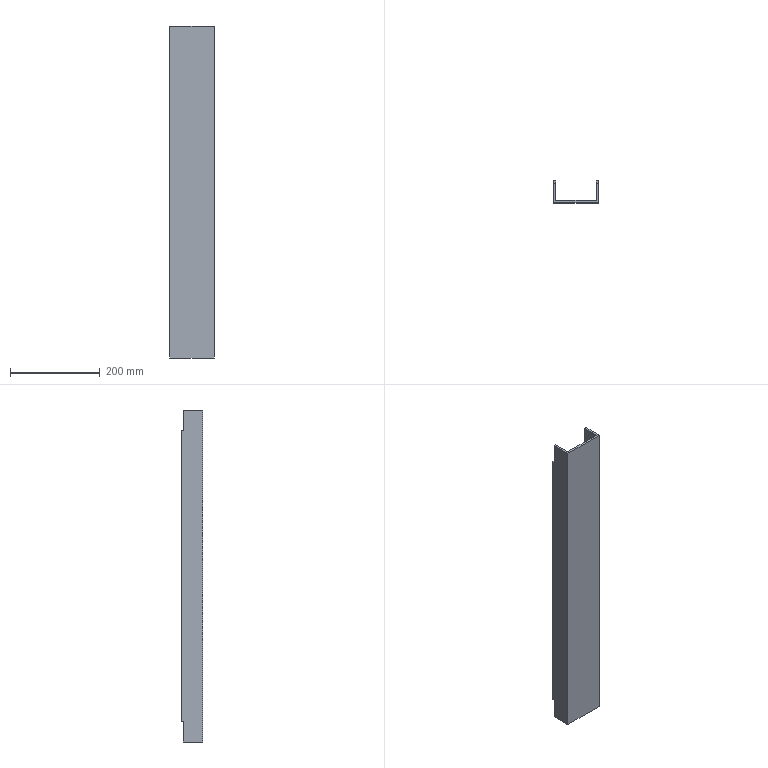Part | SolidWorks | features ICE 6, Cut 4, Extrusion 1 | 1 solid | 18 faces | box 100 x 48 x 740 mm | volume 683700 mm3 | plane 18
STEP:
#1=CARTESIAN_POINT('',(100.,48.,695.));
#2=VERTEX_POINT('',#1);
#3=CARTESIAN_POINT('',(100.,48.,45.));
#4=VERTEX_POINT('',#3);
#5=CARTESIAN_POINT('',(100.,48.,740.));
#6=DIRECTION('',(0.,0.,-1.));
#7=VECTOR('',#6,1000.);
#8=LINE('',#5,#7);
#9=EDGE_CURVE('',#2,#4,#8,.T.);
#10=ORIENTED_EDGE('',*,*,#9,.T.);
#11=CARTESIAN_POINT('',(95.,48.,45.));
#12=VERTEX_POINT('',#11);
#13=CARTESIAN_POINT('',(95.,48.,45.));
#14=DIRECTION('',(1.,0.,0.));
#15=VECTOR('',#14,1000.);
#16=LINE('',#13,#15);
#17=EDGE_CURVE('',#12,#4,#16,.T.);
#18=ORIENTED_EDGE('',*,*,#17,.F.);
#19=CARTESIAN_POINT('',(95.,48.,695.));
#20=VERTEX_POINT('',#19);
#21=CARTESIAN_POINT('',(95.,48.,740.));
#22=DIRECTION('',(0.,0.,-1.));
#23=VECTOR('',#22,1000.);
#24=LINE('',#21,#23);
#25=EDGE_CURVE('',#20,#12,#24,.T.);
#26=ORIENTED_EDGE('',*,*,#25,.F.);
#27=CARTESIAN_POINT('',(100.,48.,695.));
#28=DIRECTION('',(-1.,0.,0.));
#29=VECTOR('',#28,1000.);
#30=LINE('',#27,#29);
#31=EDGE_CURVE('',#2,#20,#30,.T.);
#32=ORIENTED_EDGE('',*,*,#31,.F.);
#33=EDGE_LOOP('',(#10,#18,#26,#32));
#34=FACE_OUTER_BOUND('',#33,.T.);
#35=CARTESIAN_POINT('',(95.,48.,740.));
#36=DIRECTION('',(0.,-1.,0.));
#37=DIRECTION('',(0.,0.,-1.));
#38=AXIS2_PLACEMENT_3D('',#35,#36,#37);
#39=PLANE('',#38);
#40=ADVANCED_FACE('',(#34),#39,.F.);
#41=CARTESIAN_POINT('',(5.,48.,695.));
#42=VERTEX_POINT('',#41);
#43=CARTESIAN_POINT('',(5.,48.,45.));
#44=VERTEX_POINT('',#43);
#45=CARTESIAN_POINT('',(5.,48.,740.));
#46=DIRECTION('',(0.,0.,-1.));
#47=VECTOR('',#46,1000.);
#48=LINE('',#45,#47);
#49=EDGE_CURVE('',#42,#44,#48,.T.);
#50=ORIENTED_EDGE('',*,*,#49,.T.);
#51=CARTESIAN_POINT('',(0.,48.,45.));
#52=VERTEX_POINT('',#51);
#53=CARTESIAN_POINT('',(0.,48.,45.));
#54=DIRECTION('',(1.,0.,0.));
#55=VECTOR('',#54,1000.);
#56=LINE('',#53,#55);
#57=EDGE_CURVE('',#52,#44,#56,.T.);
#58=ORIENTED_EDGE('',*,*,#57,.F.);
#59=CARTESIAN_POINT('',(0.,48.,695.));
#60=VERTEX_POINT('',#59);
#61=CARTESIAN_POINT('',(0.,48.,740.));
#62=DIRECTION('',(0.,0.,-1.));
#63=VECTOR('',#62,1000.);
#64=LINE('',#61,#63);
#65=EDGE_CURVE('',#60,#52,#64,.T.);
#66=ORIENTED_EDGE('',*,*,#65,.F.);
#67=CARTESIAN_POINT('',(5.,48.,695.));
#68=DIRECTION('',(-1.,0.,0.));
#69=VECTOR('',#68,1000.);
#70=LINE('',#67,#69);
#71=EDGE_CURVE('',#42,#60,#70,.T.);
#72=ORIENTED_EDGE('',*,*,#71,.F.);
#73=EDGE_LOOP('',(#50,#58,#66,#72));
#74=FACE_OUTER_BOUND('',#73,.T.);
#75=CARTESIAN_POINT('',(0.,48.,740.));
#76=DIRECTION('',(0.,-1.,0.));
#77=DIRECTION('',(0.,0.,-1.));
#78=AXIS2_PLACEMENT_3D('',#75,#76,#77);
#79=PLANE('',#78);
#80=ADVANCED_FACE('',(#74),#79,.F.);
#81=CARTESIAN_POINT('',(0.,43.,695.));
#82=VERTEX_POINT('',#81);
#83=CARTESIAN_POINT('',(0.,43.,740.));
#84=VERTEX_POINT('',#83);
#85=CARTESIAN_POINT('',(0.,43.,695.));
#86=DIRECTION('',(0.,0.,1.));
#87=VECTOR('',#86,1000.);
#88=LINE('',#85,#87);
#89=EDGE_CURVE('',#82,#84,#88,.T.);
#90=ORIENTED_EDGE('',*,*,#89,.F.);
#91=CARTESIAN_POINT('',(0.,48.,695.));
#92=DIRECTION('',(0.,-1.,0.));
#93=VECTOR('',#92,1000.);
#94=LINE('',#91,#93);
#95=EDGE_CURVE('',#60,#82,#94,.T.);
#96=ORIENTED_EDGE('',*,*,#95,.F.);
#97=ORIENTED_EDGE('',*,*,#65,.T.);
#98=CARTESIAN_POINT('',(0.,43.,45.));
#99=VERTEX_POINT('',#98);
#100=CARTESIAN_POINT('',(0.,43.,45.));
#101=DIRECTION('',(0.,1.,0.));
#102=VECTOR('',#101,1000.);
#103=LINE('',#100,#102);
#104=EDGE_CURVE('',#99,#52,#103,.T.);
#105=ORIENTED_EDGE('',*,*,#104,.F.);
#106=CARTESIAN_POINT('',(0.,43.,0.));
#107=VERTEX_POINT('',#106);
#108=CARTESIAN_POINT('',(0.,43.,45.));
#109=DIRECTION('',(0.,0.,-1.));
#110=VECTOR('',#109,1000.);
#111=LINE('',#108,#110);
#112=EDGE_CURVE('',#99,#107,#111,.T.);
#113=ORIENTED_EDGE('',*,*,#112,.T.);
#114=CARTESIAN_POINT('',(0.,0.,0.));
#115=VERTEX_POINT('',#114);
#116=CARTESIAN_POINT('',(0.,0.,0.));
#117=DIRECTION('',(0.,1.,0.));
#118=VECTOR('',#117,1000.);
#119=LINE('',#116,#118);
#120=EDGE_CURVE('',#115,#107,#119,.T.);
#121=ORIENTED_EDGE('',*,*,#120,.F.);
#122=CARTESIAN_POINT('',(0.,0.,740.));
#123=VERTEX_POINT('',#122);
#124=CARTESIAN_POINT('',(0.,0.,740.));
#125=DIRECTION('',(0.,0.,-1.));
#126=VECTOR('',#125,1000.);
#127=LINE('',#124,#126);
#128=EDGE_CURVE('',#123,#115,#127,.T.);
#129=ORIENTED_EDGE('',*,*,#128,.F.);
#130=CARTESIAN_POINT('',(0.,43.,740.));
#131=DIRECTION('',(0.,-1.,0.));
#132=VECTOR('',#131,1000.);
#133=LINE('',#130,#132);
#134=EDGE_CURVE('',#84,#123,#133,.T.);
#135=ORIENTED_EDGE('',*,*,#134,.F.);
#136=EDGE_LOOP('',(#90,#96,#97,#105,#113,#121,#129,#135));
#137=FACE_OUTER_BOUND('',#136,.T.);
#138=CARTESIAN_POINT('',(0.,0.,740.));
#139=DIRECTION('',(1.,0.,0.));
#140=DIRECTION('',(0.,0.,-1.));
#141=AXIS2_PLACEMENT_3D('',#138,#139,#140);
#142=PLANE('',#141);
#143=ADVANCED_FACE('',(#137),#142,.F.);
#144=CARTESIAN_POINT('',(100.,0.,740.));
#145=VERTEX_POINT('',#144);
#146=CARTESIAN_POINT('',(100.,0.,0.));
#147=VERTEX_POINT('',#146);
#148=CARTESIAN_POINT('',(100.,0.,740.));
#149=DIRECTION('',(0.,0.,-1.));
#150=VECTOR('',#149,1000.);
#151=LINE('',#148,#150);
#152=EDGE_CURVE('',#145,#147,#151,.T.);
#153=ORIENTED_EDGE('',*,*,#152,.F.);
#154=CARTESIAN_POINT('',(0.,0.,740.));
#155=DIRECTION('',(1.,0.,0.));
#156=VECTOR('',#155,1000.);
#157=LINE('',#154,#156);
#158=EDGE_CURVE('',#123,#145,#157,.T.);
#159=ORIENTED_EDGE('',*,*,#158,.F.);
#160=ORIENTED_EDGE('',*,*,#128,.T.);
#161=CARTESIAN_POINT('',(100.,0.,0.));
#162=DIRECTION('',(-1.,0.,0.));
#163=VECTOR('',#162,1000.);
#164=LINE('',#161,#163);
#165=EDGE_CURVE('',#147,#115,#164,.T.);
#166=ORIENTED_EDGE('',*,*,#165,.F.);
#167=EDGE_LOOP('',(#153,#159,#160,#166));
#168=FACE_OUTER_BOUND('',#167,.T.);
#169=CARTESIAN_POINT('',(0.,0.,740.));
#170=DIRECTION('',(0.,1.,0.));
#171=DIRECTION('',(0.,0.,1.));
#172=AXIS2_PLACEMENT_3D('',#169,#170,#171);
#173=PLANE('',#172);
#174=ADVANCED_FACE('',(#168),#173,.F.);
#175=CARTESIAN_POINT('',(100.,43.,695.));
#176=VERTEX_POINT('',#175);
#177=CARTESIAN_POINT('',(100.,43.,695.));
#178=DIRECTION('',(0.,1.,0.));
#179=VECTOR('',#178,1000.);
#180=LINE('',#177,#179);
#181=EDGE_CURVE('',#176,#2,#180,.T.);
#182=ORIENTED_EDGE('',*,*,#181,.F.);
#183=CARTESIAN_POINT('',(100.,43.,740.));
#184=VERTEX_POINT('',#183);
#185=CARTESIAN_POINT('',(100.,43.,695.));
#186=DIRECTION('',(0.,0.,1.));
#187=VECTOR('',#186,1000.);
#188=LINE('',#185,#187);
#189=EDGE_CURVE('',#176,#184,#188,.T.);
#190=ORIENTED_EDGE('',*,*,#189,.T.);
#191=CARTESIAN_POINT('',(100.,0.,740.));
#192=DIRECTION('',(0.,1.,0.));
#193=VECTOR('',#192,1000.);
#194=LINE('',#191,#193);
#195=EDGE_CURVE('',#145,#184,#194,.T.);
#196=ORIENTED_EDGE('',*,*,#195,.F.);
#197=ORIENTED_EDGE('',*,*,#152,.T.);
#198=CARTESIAN_POINT('',(100.,43.,0.));
#199=VERTEX_POINT('',#198);
#200=CARTESIAN_POINT('',(100.,43.,0.));
#201=DIRECTION('',(0.,-1.,0.));
#202=VECTOR('',#201,1000.);
#203=LINE('',#200,#202);
#204=EDGE_CURVE('',#199,#147,#203,.T.);
#205=ORIENTED_EDGE('',*,*,#204,.F.);
#206=CARTESIAN_POINT('',(100.,43.,45.));
#207=VERTEX_POINT('',#206);
#208=CARTESIAN_POINT('',(100.,43.,45.));
#209=DIRECTION('',(0.,0.,-1.));
#210=VECTOR('',#209,1000.);
#211=LINE('',#208,#210);
#212=EDGE_CURVE('',#207,#199,#211,.T.);
#213=ORIENTED_EDGE('',*,*,#212,.F.);
#214=CARTESIAN_POINT('',(100.,48.,45.));
#215=DIRECTION('',(0.,-1.,0.));
#216=VECTOR('',#215,1000.);
#217=LINE('',#214,#216);
#218=EDGE_CURVE('',#4,#207,#217,.T.);
#219=ORIENTED_EDGE('',*,*,#218,.F.);
#220=ORIENTED_EDGE('',*,*,#9,.F.);
#221=EDGE_LOOP('',(#182,#190,#196,#197,#205,#213,#219,#220));
#222=FACE_OUTER_BOUND('',#221,.T.);
#223=CARTESIAN_POINT('',(100.,0.,740.));
#224=DIRECTION('',(-1.,0.,0.));
#225=DIRECTION('',(0.,0.,1.));
#226=AXIS2_PLACEMENT_3D('',#223,#224,#225);
#227=PLANE('',#226);
#228=ADVANCED_FACE('',(#222),#227,.F.);
#229=CARTESIAN_POINT('',(95.,43.,45.));
#230=VERTEX_POINT('',#229);
#231=CARTESIAN_POINT('',(95.,43.,45.));
#232=DIRECTION('',(0.,1.,0.));
#233=VECTOR('',#232,1000.);
#234=LINE('',#231,#233);
#235=EDGE_CURVE('',#230,#12,#234,.T.);
#236=ORIENTED_EDGE('',*,*,#235,.F.);
#237=CARTESIAN_POINT('',(95.,43.,0.));
#238=VERTEX_POINT('',#237);
#239=CARTESIAN_POINT('',(95.,43.,740.));
#240=DIRECTION('',(0.,0.,-1.));
#241=VECTOR('',#240,1000.);
#242=LINE('',#239,#241);
#243=EDGE_CURVE('',#230,#238,#242,.T.);
#244=ORIENTED_EDGE('',*,*,#243,.T.);
#245=CARTESIAN_POINT('',(95.,5.,0.));
#246=VERTEX_POINT('',#245);
#247=CARTESIAN_POINT('',(95.,5.,0.));
#248=DIRECTION('',(0.,1.,0.));
#249=VECTOR('',#248,1000.);
#250=LINE('',#247,#249);
#251=EDGE_CURVE('',#246,#238,#250,.T.);
#252=ORIENTED_EDGE('',*,*,#251,.F.);
#253=CARTESIAN_POINT('',(95.,5.,740.));
#254=VERTEX_POINT('',#253);
#255=CARTESIAN_POINT('',(95.,5.,740.));
#256=DIRECTION('',(0.,0.,-1.));
#257=VECTOR('',#256,1000.);
#258=LINE('',#255,#257);
#259=EDGE_CURVE('',#254,#246,#258,.T.);
#260=ORIENTED_EDGE('',*,*,#259,.F.);
#261=CARTESIAN_POINT('',(95.,43.,740.));
#262=VERTEX_POINT('',#261);
#263=CARTESIAN_POINT('',(95.,43.,740.));
#264=DIRECTION('',(0.,-1.,0.));
#265=VECTOR('',#264,1000.);
#266=LINE('',#263,#265);
#267=EDGE_CURVE('',#262,#254,#266,.T.);
#268=ORIENTED_EDGE('',*,*,#267,.F.);
#269=CARTESIAN_POINT('',(95.,43.,695.));
#270=VERTEX_POINT('',#269);
#271=CARTESIAN_POINT('',(95.,43.,740.));
#272=DIRECTION('',(0.,0.,-1.));
#273=VECTOR('',#272,1000.);
#274=LINE('',#271,#273);
#275=EDGE_CURVE('',#262,#270,#274,.T.);
#276=ORIENTED_EDGE('',*,*,#275,.T.);
#277=CARTESIAN_POINT('',(95.,48.,695.));
#278=DIRECTION('',(0.,-1.,0.));
#279=VECTOR('',#278,1000.);
#280=LINE('',#277,#279);
#281=EDGE_CURVE('',#20,#270,#280,.T.);
#282=ORIENTED_EDGE('',*,*,#281,.F.);
#283=ORIENTED_EDGE('',*,*,#25,.T.);
#284=EDGE_LOOP('',(#236,#244,#252,#260,#268,#276,#282,#283));
#285=FACE_OUTER_BOUND('',#284,.T.);
#286=CARTESIAN_POINT('',(95.,5.,740.));
#287=DIRECTION('',(1.,0.,0.));
#288=DIRECTION('',(0.,0.,-1.));
#289=AXIS2_PLACEMENT_3D('',#286,#287,#288);
#290=PLANE('',#289);
#291=ADVANCED_FACE('',(#285),#290,.F.);
#292=CARTESIAN_POINT('',(5.,5.,740.));
#293=VERTEX_POINT('',#292);
#294=CARTESIAN_POINT('',(5.,5.,0.));
#295=VERTEX_POINT('',#294);
#296=CARTESIAN_POINT('',(5.,5.,740.));
#297=DIRECTION('',(0.,0.,-1.));
#298=VECTOR('',#297,1000.);
#299=LINE('',#296,#298);
#300=EDGE_CURVE('',#293,#295,#299,.T.);
#301=ORIENTED_EDGE('',*,*,#300,.F.);
#302=CARTESIAN_POINT('',(95.,5.,740.));
#303=DIRECTION('',(-1.,0.,0.));
#304=VECTOR('',#303,1000.);
#305=LINE('',#302,#304);
#306=EDGE_CURVE('',#254,#293,#305,.T.);
#307=ORIENTED_EDGE('',*,*,#306,.F.);
#308=ORIENTED_EDGE('',*,*,#259,.T.);
#309=CARTESIAN_POINT('',(5.,5.,0.));
#310=DIRECTION('',(1.,0.,0.));
#311=VECTOR('',#310,1000.);
#312=LINE('',#309,#311);
#313=EDGE_CURVE('',#295,#246,#312,.T.);
#314=ORIENTED_EDGE('',*,*,#313,.F.);
#315=EDGE_LOOP('',(#301,#307,#308,#314));
#316=FACE_OUTER_BOUND('',#315,.T.);
#317=CARTESIAN_POINT('',(5.,5.,740.));
#318=DIRECTION('',(0.,-1.,0.));
#319=DIRECTION('',(0.,0.,-1.));
#320=AXIS2_PLACEMENT_3D('',#317,#318,#319);
#321=PLANE('',#320);
#322=ADVANCED_FACE('',(#316),#321,.F.);
#323=CARTESIAN_POINT('',(5.,43.,695.));
#324=VERTEX_POINT('',#323);
#325=CARTESIAN_POINT('',(5.,43.,695.));
#326=DIRECTION('',(0.,1.,0.));
#327=VECTOR('',#326,1000.);
#328=LINE('',#325,#327);
#329=EDGE_CURVE('',#324,#42,#328,.T.);
#330=ORIENTED_EDGE('',*,*,#329,.F.);
#331=CARTESIAN_POINT('',(5.,43.,740.));
#332=VERTEX_POINT('',#331);
#333=CARTESIAN_POINT('',(5.,43.,740.));
#334=DIRECTION('',(0.,0.,1.));
#335=VECTOR('',#334,1000.);
#336=LINE('',#333,#335);
#337=EDGE_CURVE('',#324,#332,#336,.T.);
#338=ORIENTED_EDGE('',*,*,#337,.T.);
#339=CARTESIAN_POINT('',(5.,5.,740.));
#340=DIRECTION('',(0.,1.,0.));
#341=VECTOR('',#340,1000.);
#342=LINE('',#339,#341);
#343=EDGE_CURVE('',#293,#332,#342,.T.);
#344=ORIENTED_EDGE('',*,*,#343,.F.);
#345=ORIENTED_EDGE('',*,*,#300,.T.);
#346=CARTESIAN_POINT('',(5.,43.,0.));
#347=VERTEX_POINT('',#346);
#348=CARTESIAN_POINT('',(5.,43.,0.));
#349=DIRECTION('',(0.,-1.,0.));
#350=VECTOR('',#349,1000.);
#351=LINE('',#348,#350);
#352=EDGE_CURVE('',#347,#295,#351,.T.);
#353=ORIENTED_EDGE('',*,*,#352,.F.);
#354=CARTESIAN_POINT('',(5.,43.,45.));
#355=VERTEX_POINT('',#354);
#356=CARTESIAN_POINT('',(5.,43.,740.));
#357=DIRECTION('',(0.,0.,1.));
#358=VECTOR('',#357,1000.);
#359=LINE('',#356,#358);
#360=EDGE_CURVE('',#347,#355,#359,.T.);
#361=ORIENTED_EDGE('',*,*,#360,.T.);
#362=CARTESIAN_POINT('',(5.,48.,45.));
#363=DIRECTION('',(0.,-1.,0.));
#364=VECTOR('',#363,1000.);
#365=LINE('',#362,#364);
#366=EDGE_CURVE('',#44,#355,#365,.T.);
#367=ORIENTED_EDGE('',*,*,#366,.F.);
#368=ORIENTED_EDGE('',*,*,#49,.F.);
#369=EDGE_LOOP('',(#330,#338,#344,#345,#353,#361,#367,#368));
#370=FACE_OUTER_BOUND('',#369,.T.);
#371=CARTESIAN_POINT('',(5.,5.,740.));
#372=DIRECTION('',(-1.,0.,0.));
#373=DIRECTION('',(0.,0.,1.));
#374=AXIS2_PLACEMENT_3D('',#371,#372,#373);
#375=PLANE('',#374);
#376=ADVANCED_FACE('',(#370),#375,.F.);
#377=ORIENTED_EDGE('',*,*,#337,.F.);
#378=CARTESIAN_POINT('',(0.,43.,695.));
#379=DIRECTION('',(1.,0.,0.));
#380=VECTOR('',#379,1000.);
#381=LINE('',#378,#380);
#382=EDGE_CURVE('',#82,#324,#381,.T.);
#383=ORIENTED_EDGE('',*,*,#382,.F.);
#384=ORIENTED_EDGE('',*,*,#89,.T.);
#385=CARTESIAN_POINT('',(5.,43.,740.));
#386=DIRECTION('',(-1.,0.,0.));
#387=VECTOR('',#386,1000.);
#388=LINE('',#385,#387);
#389=EDGE_CURVE('',#332,#84,#388,.T.);
#390=ORIENTED_EDGE('',*,*,#389,.F.);
#391=EDGE_LOOP('',(#377,#383,#384,#390));
#392=FACE_OUTER_BOUND('',#391,.T.);
#393=CARTESIAN_POINT('',(0.,43.,695.));
#394=DIRECTION('',(0.,-1.,0.));
#395=DIRECTION('',(0.,0.,-1.));
#396=AXIS2_PLACEMENT_3D('',#393,#394,#395);
#397=PLANE('',#396);
#398=ADVANCED_FACE('',(#392),#397,.F.);
#399=ORIENTED_EDGE('',*,*,#189,.F.);
#400=CARTESIAN_POINT('',(95.,43.,695.));
#401=DIRECTION('',(1.,0.,0.));
#402=VECTOR('',#401,1000.);
#403=LINE('',#400,#402);
#404=EDGE_CURVE('',#270,#176,#403,.T.);
#405=ORIENTED_EDGE('',*,*,#404,.F.);
#406=ORIENTED_EDGE('',*,*,#275,.F.);
#407=CARTESIAN_POINT('',(100.,43.,740.));
#408=DIRECTION('',(-1.,0.,0.));
#409=VECTOR('',#408,1000.);
#410=LINE('',#407,#409);
#411=EDGE_CURVE('',#184,#262,#410,.T.);
#412=ORIENTED_EDGE('',*,*,#411,.F.);
#413=EDGE_LOOP('',(#399,#405,#406,#412));
#414=FACE_OUTER_BOUND('',#413,.T.);
#415=CARTESIAN_POINT('',(0.,43.,695.));
#416=DIRECTION('',(0.,-1.,0.));
#417=DIRECTION('',(0.,0.,-1.));
#418=AXIS2_PLACEMENT_3D('',#415,#416,#417);
#419=PLANE('',#418);
#420=ADVANCED_FACE('',(#414),#419,.F.);
#421=ORIENTED_EDGE('',*,*,#112,.F.);
#422=CARTESIAN_POINT('',(5.,43.,45.));
#423=DIRECTION('',(-1.,0.,0.));
#424=VECTOR('',#423,1000.);
#425=LINE('',#422,#424);
#426=EDGE_CURVE('',#355,#99,#425,.T.);
#427=ORIENTED_EDGE('',*,*,#426,.F.);
#428=ORIENTED_EDGE('',*,*,#360,.F.);
#429=CARTESIAN_POINT('',(0.,43.,0.));
#430=DIRECTION('',(1.,0.,0.));
#431=VECTOR('',#430,1000.);
#432=LINE('',#429,#431);
#433=EDGE_CURVE('',#107,#347,#432,.T.);
#434=ORIENTED_EDGE('',*,*,#433,.F.);
#435=EDGE_LOOP('',(#421,#427,#428,#434));
#436=FACE_OUTER_BOUND('',#435,.T.);
#437=CARTESIAN_POINT('',(100.,43.,45.));
#438=DIRECTION('',(0.,-1.,0.));
#439=DIRECTION('',(0.,0.,-1.));
#440=AXIS2_PLACEMENT_3D('',#437,#438,#439);
#441=PLANE('',#440);
#442=ADVANCED_FACE('',(#436),#441,.F.);
#443=ORIENTED_EDGE('',*,*,#243,.F.);
#444=CARTESIAN_POINT('',(100.,43.,45.));
#445=DIRECTION('',(-1.,0.,0.));
#446=VECTOR('',#445,1000.);
#447=LINE('',#444,#446);
#448=EDGE_CURVE('',#207,#230,#447,.T.);
#449=ORIENTED_EDGE('',*,*,#448,.F.);
#450=ORIENTED_EDGE('',*,*,#212,.T.);
#451=CARTESIAN_POINT('',(95.,43.,0.));
#452=DIRECTION('',(1.,0.,0.));
#453=VECTOR('',#452,1000.);
#454=LINE('',#451,#453);
#455=EDGE_CURVE('',#238,#199,#454,.T.);
#456=ORIENTED_EDGE('',*,*,#455,.F.);
#457=EDGE_LOOP('',(#443,#449,#450,#456));
#458=FACE_OUTER_BOUND('',#457,.T.);
#459=CARTESIAN_POINT('',(100.,43.,45.));
#460=DIRECTION('',(0.,-1.,0.));
#461=DIRECTION('',(0.,0.,-1.));
#462=AXIS2_PLACEMENT_3D('',#459,#460,#461);
#463=PLANE('',#462);
#464=ADVANCED_FACE('',(#458),#463,.F.);
#465=ORIENTED_EDGE('',*,*,#313,.T.);
#466=ORIENTED_EDGE('',*,*,#251,.T.);
#467=ORIENTED_EDGE('',*,*,#455,.T.);
#468=ORIENTED_EDGE('',*,*,#204,.T.);
#469=ORIENTED_EDGE('',*,*,#165,.T.);
#470=ORIENTED_EDGE('',*,*,#120,.T.);
#471=ORIENTED_EDGE('',*,*,#433,.T.);
#472=ORIENTED_EDGE('',*,*,#352,.T.);
#473=EDGE_LOOP('',(#465,#466,#467,#468,#469,#470,#471,#472));
#474=FACE_OUTER_BOUND('',#473,.T.);
#475=CARTESIAN_POINT('',(0.,0.,0.));
#476=DIRECTION('',(0.,0.,1.));
#477=DIRECTION('',(1.,0.,0.));
#478=AXIS2_PLACEMENT_3D('',#475,#476,#477);
#479=PLANE('',#478);
#480=ADVANCED_FACE('',(#474),#479,.F.);
#481=ORIENTED_EDGE('',*,*,#104,.T.);
#482=ORIENTED_EDGE('',*,*,#57,.T.);
#483=ORIENTED_EDGE('',*,*,#366,.T.);
#484=ORIENTED_EDGE('',*,*,#426,.T.);
#485=EDGE_LOOP('',(#481,#482,#483,#484));
#486=FACE_OUTER_BOUND('',#485,.T.);
#487=CARTESIAN_POINT('',(0.,0.,45.));
#488=DIRECTION('',(0.,0.,-1.));
#489=DIRECTION('',(-1.,0.,0.));
#490=AXIS2_PLACEMENT_3D('',#487,#488,#489);
#491=PLANE('',#490);
#492=ADVANCED_FACE('',(#486),#491,.T.);
#493=ORIENTED_EDGE('',*,*,#218,.T.);
#494=ORIENTED_EDGE('',*,*,#448,.T.);
#495=ORIENTED_EDGE('',*,*,#235,.T.);
#496=ORIENTED_EDGE('',*,*,#17,.T.);
#497=EDGE_LOOP('',(#493,#494,#495,#496));
#498=FACE_OUTER_BOUND('',#497,.T.);
#499=CARTESIAN_POINT('',(0.,0.,45.));
#500=DIRECTION('',(0.,0.,-1.));
#501=DIRECTION('',(-1.,0.,0.));
#502=AXIS2_PLACEMENT_3D('',#499,#500,#501);
#503=PLANE('',#502);
#504=ADVANCED_FACE('',(#498),#503,.T.);
#505=ORIENTED_EDGE('',*,*,#134,.T.);
#506=ORIENTED_EDGE('',*,*,#158,.T.);
#507=ORIENTED_EDGE('',*,*,#195,.T.);
#508=ORIENTED_EDGE('',*,*,#411,.T.);
#509=ORIENTED_EDGE('',*,*,#267,.T.);
#510=ORIENTED_EDGE('',*,*,#306,.T.);
#511=ORIENTED_EDGE('',*,*,#343,.T.);
#512=ORIENTED_EDGE('',*,*,#389,.T.);
#513=EDGE_LOOP('',(#505,#506,#507,#508,#509,#510,#511,#512));
#514=FACE_OUTER_BOUND('',#513,.T.);
#515=CARTESIAN_POINT('',(0.,0.,740.));
#516=DIRECTION('',(0.,0.,1.));
#517=DIRECTION('',(1.,0.,0.));
#518=AXIS2_PLACEMENT_3D('',#515,#516,#517);
#519=PLANE('',#518);
#520=ADVANCED_FACE('',(#514),#519,.T.);
#521=ORIENTED_EDGE('',*,*,#95,.T.);
#522=ORIENTED_EDGE('',*,*,#382,.T.);
#523=ORIENTED_EDGE('',*,*,#329,.T.);
#524=ORIENTED_EDGE('',*,*,#71,.T.);
#525=EDGE_LOOP('',(#521,#522,#523,#524));
#526=FACE_OUTER_BOUND('',#525,.T.);
#527=CARTESIAN_POINT('',(0.,0.,695.));
#528=DIRECTION('',(0.,0.,1.));
#529=DIRECTION('',(1.,0.,0.));
#530=AXIS2_PLACEMENT_3D('',#527,#528,#529);
#531=PLANE('',#530);
#532=ADVANCED_FACE('',(#526),#531,.T.);
#533=ORIENTED_EDGE('',*,*,#181,.T.);
#534=ORIENTED_EDGE('',*,*,#31,.T.);
#535=ORIENTED_EDGE('',*,*,#281,.T.);
#536=ORIENTED_EDGE('',*,*,#404,.T.);
#537=EDGE_LOOP('',(#533,#534,#535,#536));
#538=FACE_OUTER_BOUND('',#537,.T.);
#539=CARTESIAN_POINT('',(0.,0.,695.));
#540=DIRECTION('',(0.,0.,1.));
#541=DIRECTION('',(1.,0.,0.));
#542=AXIS2_PLACEMENT_3D('',#539,#540,#541);
#543=PLANE('',#542);
#544=ADVANCED_FACE('',(#538),#543,.T.);
#545=CLOSED_SHELL('',(#40,#80,#143,#174,#228,#291,#322,#376,#398,#420,#442,#464,#480,#492,#504,#520,#532,#544));
#546=MANIFOLD_SOLID_BREP('',#545);
#547=CARTESIAN_POINT('',(0.,0.,0.));
#548=DIRECTION('',(0.,0.,1.));
#549=DIRECTION('',(1.,0.,0.));
#550=AXIS2_PLACEMENT_3D('',#547,#548,#549);
#551=(LENGTH_UNIT()NAMED_UNIT(*)SI_UNIT(.MILLI.,.METRE.));
#552=UNCERTAINTY_MEASURE_WITH_UNIT(LENGTH_MEASURE(0.00001),#551,'','');
#553=(NAMED_UNIT(*)PLANE_ANGLE_UNIT()SI_UNIT($,.RADIAN.));
#554=(NAMED_UNIT(*)SI_UNIT($,.STERADIAN.)SOLID_ANGLE_UNIT());
#555=(GEOMETRIC_REPRESENTATION_CONTEXT(3)GLOBAL_UNCERTAINTY_ASSIGNED_CONTEXT((#552))GLOBAL_UNIT_ASSIGNED_CONTEXT((#551,#553,#554))REPRESENTATION_CONTEXT('',''));
#556=ADVANCED_BREP_SHAPE_REPRESENTATION('',(#546,#550),#555);